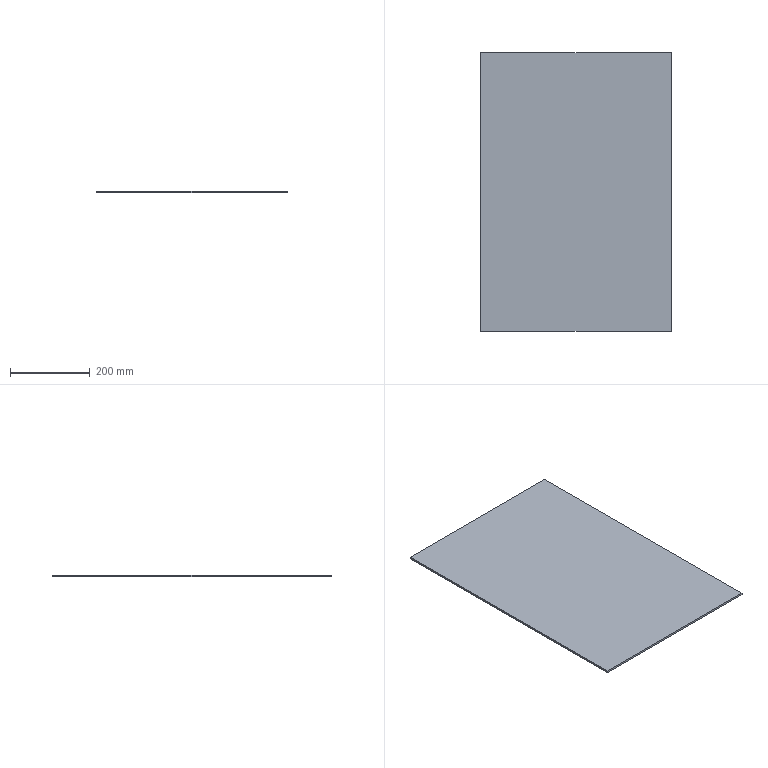Part | STEP file | 001-002-Face Plate-2 | 1 solid | 6 faces | box 478 x 698 x 5 mm | volume 1668220 mm3 | plane 6
STEP:
#1=CARTESIAN_POINT('',(0.,0.,0.));
#2=DIRECTION('',(0.,0.,1.));
#3=DIRECTION('',(1.,0.,0.));
#4=AXIS2_PLACEMENT_3D('',#1,#2,#3);
#5=CARTESIAN_POINT('',(239.,-349.,0.));
#6=VERTEX_POINT('',#5);
#7=CARTESIAN_POINT('',(239.,349.,0.));
#8=VERTEX_POINT('',#7);
#9=CARTESIAN_POINT('',(239.,-349.,0.));
#10=DIRECTION('',(0.,1.,0.));
#11=VECTOR('',#10,1.);
#12=LINE('',#9,#11);
#13=CARTESIAN_POINT('',(239.,-349.,5.));
#14=DIRECTION('',(-1.,0.,0.));
#15=DIRECTION('',(0.,0.,1.));
#16=AXIS2_PLACEMENT_3D('',#13,#14,#15);
#17=PLANE('',#16);
#18=CARTESIAN_POINT('',(-5.,0.));
#19=DIRECTION('',(0.,1.));
#20=VECTOR('',#19,1.);
#21=LINE('',#18,#20);
#22=(GEOMETRIC_REPRESENTATION_CONTEXT(2)PARAMETRIC_REPRESENTATION_CONTEXT()REPRESENTATION_CONTEXT('',''));
#23=DEFINITIONAL_REPRESENTATION('',(#21),#22);
#24=PCURVE('',#17,#23);
#25=CARTESIAN_POINT('',(0.,0.,0.));
#26=DIRECTION('',(0.,0.,-1.));
#27=DIRECTION('',(-1.,0.,0.));
#28=AXIS2_PLACEMENT_3D('',#25,#26,#27);
#29=PLANE('',#28);
#30=CARTESIAN_POINT('',(-239.,-349.));
#31=DIRECTION('',(0.,1.));
#32=VECTOR('',#31,1.);
#33=LINE('',#30,#32);
#34=(GEOMETRIC_REPRESENTATION_CONTEXT(2)PARAMETRIC_REPRESENTATION_CONTEXT()REPRESENTATION_CONTEXT('',''));
#35=DEFINITIONAL_REPRESENTATION('',(#33),#34);
#36=PCURVE('',#29,#35);
#37=SURFACE_CURVE('',#12,(#24,#36),.PCURVE_S1.);
#38=EDGE_CURVE('',#6,#8,#37,.T.);
#39=ORIENTED_EDGE('',*,*,#38,.T.);
#40=CARTESIAN_POINT('',(239.,349.,5.));
#41=VERTEX_POINT('',#40);
#42=CARTESIAN_POINT('',(239.,349.,5.));
#43=DIRECTION('',(0.,0.,-1.));
#44=VECTOR('',#43,1.);
#45=LINE('',#42,#44);
#46=CARTESIAN_POINT('',(0.,698.));
#47=DIRECTION('',(-1.,0.));
#48=VECTOR('',#47,1.);
#49=LINE('',#46,#48);
#50=(GEOMETRIC_REPRESENTATION_CONTEXT(2)PARAMETRIC_REPRESENTATION_CONTEXT()REPRESENTATION_CONTEXT('',''));
#51=DEFINITIONAL_REPRESENTATION('',(#49),#50);
#52=PCURVE('',#17,#51);
#53=CARTESIAN_POINT('',(-239.,349.,5.));
#54=DIRECTION('',(0.,-1.,0.));
#55=DIRECTION('',(0.,0.,-1.));
#56=AXIS2_PLACEMENT_3D('',#53,#54,#55);
#57=PLANE('',#56);
#58=CARTESIAN_POINT('',(0.,478.));
#59=DIRECTION('',(1.,0.));
#60=VECTOR('',#59,1.);
#61=LINE('',#58,#60);
#62=(GEOMETRIC_REPRESENTATION_CONTEXT(2)PARAMETRIC_REPRESENTATION_CONTEXT()REPRESENTATION_CONTEXT('',''));
#63=DEFINITIONAL_REPRESENTATION('',(#61),#62);
#64=PCURVE('',#57,#63);
#65=SURFACE_CURVE('',#45,(#52,#64),.PCURVE_S1.);
#66=EDGE_CURVE('',#41,#8,#65,.T.);
#67=ORIENTED_EDGE('',*,*,#66,.F.);
#68=CARTESIAN_POINT('',(239.,-349.,5.));
#69=VERTEX_POINT('',#68);
#70=CARTESIAN_POINT('',(239.,-349.,5.));
#71=DIRECTION('',(0.,1.,0.));
#72=VECTOR('',#71,1.);
#73=LINE('',#70,#72);
#74=CARTESIAN_POINT('',(0.,0.));
#75=DIRECTION('',(0.,1.));
#76=VECTOR('',#75,1.);
#77=LINE('',#74,#76);
#78=(GEOMETRIC_REPRESENTATION_CONTEXT(2)PARAMETRIC_REPRESENTATION_CONTEXT()REPRESENTATION_CONTEXT('',''));
#79=DEFINITIONAL_REPRESENTATION('',(#77),#78);
#80=PCURVE('',#17,#79);
#81=CARTESIAN_POINT('',(0.,0.,5.));
#82=DIRECTION('',(0.,0.,-1.));
#83=DIRECTION('',(-1.,0.,0.));
#84=AXIS2_PLACEMENT_3D('',#81,#82,#83);
#85=PLANE('',#84);
#86=CARTESIAN_POINT('',(-239.,-349.));
#87=DIRECTION('',(0.,1.));
#88=VECTOR('',#87,1.);
#89=LINE('',#86,#88);
#90=(GEOMETRIC_REPRESENTATION_CONTEXT(2)PARAMETRIC_REPRESENTATION_CONTEXT()REPRESENTATION_CONTEXT('',''));
#91=DEFINITIONAL_REPRESENTATION('',(#89),#90);
#92=PCURVE('',#85,#91);
#93=SURFACE_CURVE('',#73,(#80,#92),.PCURVE_S1.);
#94=EDGE_CURVE('',#69,#41,#93,.T.);
#95=ORIENTED_EDGE('',*,*,#94,.F.);
#96=CARTESIAN_POINT('',(239.,-349.,5.));
#97=DIRECTION('',(0.,0.,-1.));
#98=VECTOR('',#97,1.);
#99=LINE('',#96,#98);
#100=CARTESIAN_POINT('',(0.,0.));
#101=DIRECTION('',(-1.,0.));
#102=VECTOR('',#101,1.);
#103=LINE('',#100,#102);
#104=(GEOMETRIC_REPRESENTATION_CONTEXT(2)PARAMETRIC_REPRESENTATION_CONTEXT()REPRESENTATION_CONTEXT('',''));
#105=DEFINITIONAL_REPRESENTATION('',(#103),#104);
#106=PCURVE('',#17,#105);
#107=CARTESIAN_POINT('',(-239.,-349.,5.));
#108=DIRECTION('',(0.,1.,0.));
#109=DIRECTION('',(0.,0.,1.));
#110=AXIS2_PLACEMENT_3D('',#107,#108,#109);
#111=PLANE('',#110);
#112=CARTESIAN_POINT('',(0.,478.));
#113=DIRECTION('',(-1.,0.));
#114=VECTOR('',#113,1.);
#115=LINE('',#112,#114);
#116=(GEOMETRIC_REPRESENTATION_CONTEXT(2)PARAMETRIC_REPRESENTATION_CONTEXT()REPRESENTATION_CONTEXT('',''));
#117=DEFINITIONAL_REPRESENTATION('',(#115),#116);
#118=PCURVE('',#111,#117);
#119=SURFACE_CURVE('',#99,(#106,#118),.PCURVE_S1.);
#120=EDGE_CURVE('',#69,#6,#119,.T.);
#121=ORIENTED_EDGE('',*,*,#120,.T.);
#122=EDGE_LOOP('',(#39,#67,#95,#121));
#123=FACE_BOUND('',#122,.T.);
#124=ADVANCED_FACE('',(#123),#17,.F.);
#125=CARTESIAN_POINT('',(-239.,349.,0.));
#126=VERTEX_POINT('',#125);
#127=CARTESIAN_POINT('',(-239.,349.,0.));
#128=DIRECTION('',(-1.,0.,0.));
#129=VECTOR('',#128,1.);
#130=LINE('',#127,#129);
#131=CARTESIAN_POINT('',(5.,0.));
#132=DIRECTION('',(0.,-1.));
#133=VECTOR('',#132,1.);
#134=LINE('',#131,#133);
#135=(GEOMETRIC_REPRESENTATION_CONTEXT(2)PARAMETRIC_REPRESENTATION_CONTEXT()REPRESENTATION_CONTEXT('',''));
#136=DEFINITIONAL_REPRESENTATION('',(#134),#135);
#137=PCURVE('',#57,#136);
#138=CARTESIAN_POINT('',(239.,349.));
#139=DIRECTION('',(1.,0.));
#140=VECTOR('',#139,1.);
#141=LINE('',#138,#140);
#142=(GEOMETRIC_REPRESENTATION_CONTEXT(2)PARAMETRIC_REPRESENTATION_CONTEXT()REPRESENTATION_CONTEXT('',''));
#143=DEFINITIONAL_REPRESENTATION('',(#141),#142);
#144=PCURVE('',#29,#143);
#145=SURFACE_CURVE('',#130,(#137,#144),.PCURVE_S1.);
#146=EDGE_CURVE('',#8,#126,#145,.T.);
#147=ORIENTED_EDGE('',*,*,#146,.T.);
#148=CARTESIAN_POINT('',(-239.,349.,5.));
#149=VERTEX_POINT('',#148);
#150=CARTESIAN_POINT('',(-239.,349.,5.));
#151=DIRECTION('',(0.,0.,-1.));
#152=VECTOR('',#151,1.);
#153=LINE('',#150,#152);
#154=CARTESIAN_POINT('',(0.,0.));
#155=DIRECTION('',(1.,0.));
#156=VECTOR('',#155,1.);
#157=LINE('',#154,#156);
#158=(GEOMETRIC_REPRESENTATION_CONTEXT(2)PARAMETRIC_REPRESENTATION_CONTEXT()REPRESENTATION_CONTEXT('',''));
#159=DEFINITIONAL_REPRESENTATION('',(#157),#158);
#160=PCURVE('',#57,#159);
#161=CARTESIAN_POINT('',(-239.,-349.,5.));
#162=DIRECTION('',(1.,0.,0.));
#163=DIRECTION('',(0.,0.,-1.));
#164=AXIS2_PLACEMENT_3D('',#161,#162,#163);
#165=PLANE('',#164);
#166=CARTESIAN_POINT('',(0.,698.));
#167=DIRECTION('',(1.,0.));
#168=VECTOR('',#167,1.);
#169=LINE('',#166,#168);
#170=(GEOMETRIC_REPRESENTATION_CONTEXT(2)PARAMETRIC_REPRESENTATION_CONTEXT()REPRESENTATION_CONTEXT('',''));
#171=DEFINITIONAL_REPRESENTATION('',(#169),#170);
#172=PCURVE('',#165,#171);
#173=SURFACE_CURVE('',#153,(#160,#172),.PCURVE_S1.);
#174=EDGE_CURVE('',#149,#126,#173,.T.);
#175=ORIENTED_EDGE('',*,*,#174,.F.);
#176=CARTESIAN_POINT('',(-239.,349.,5.));
#177=DIRECTION('',(-1.,0.,0.));
#178=VECTOR('',#177,1.);
#179=LINE('',#176,#178);
#180=CARTESIAN_POINT('',(0.,0.));
#181=DIRECTION('',(0.,-1.));
#182=VECTOR('',#181,1.);
#183=LINE('',#180,#182);
#184=(GEOMETRIC_REPRESENTATION_CONTEXT(2)PARAMETRIC_REPRESENTATION_CONTEXT()REPRESENTATION_CONTEXT('',''));
#185=DEFINITIONAL_REPRESENTATION('',(#183),#184);
#186=PCURVE('',#57,#185);
#187=CARTESIAN_POINT('',(239.,349.));
#188=DIRECTION('',(1.,0.));
#189=VECTOR('',#188,1.);
#190=LINE('',#187,#189);
#191=(GEOMETRIC_REPRESENTATION_CONTEXT(2)PARAMETRIC_REPRESENTATION_CONTEXT()REPRESENTATION_CONTEXT('',''));
#192=DEFINITIONAL_REPRESENTATION('',(#190),#191);
#193=PCURVE('',#85,#192);
#194=SURFACE_CURVE('',#179,(#186,#193),.PCURVE_S1.);
#195=EDGE_CURVE('',#41,#149,#194,.T.);
#196=ORIENTED_EDGE('',*,*,#195,.F.);
#197=ORIENTED_EDGE('',*,*,#66,.T.);
#198=EDGE_LOOP('',(#147,#175,#196,#197));
#199=FACE_BOUND('',#198,.T.);
#200=ADVANCED_FACE('',(#199),#57,.F.);
#201=CARTESIAN_POINT('',(-239.,-349.,0.));
#202=VERTEX_POINT('',#201);
#203=CARTESIAN_POINT('',(-239.,-349.,0.));
#204=DIRECTION('',(0.,-1.,0.));
#205=VECTOR('',#204,1.);
#206=LINE('',#203,#205);
#207=CARTESIAN_POINT('',(5.,0.));
#208=DIRECTION('',(0.,-1.));
#209=VECTOR('',#208,1.);
#210=LINE('',#207,#209);
#211=(GEOMETRIC_REPRESENTATION_CONTEXT(2)PARAMETRIC_REPRESENTATION_CONTEXT()REPRESENTATION_CONTEXT('',''));
#212=DEFINITIONAL_REPRESENTATION('',(#210),#211);
#213=PCURVE('',#165,#212);
#214=CARTESIAN_POINT('',(239.,-349.));
#215=DIRECTION('',(0.,-1.));
#216=VECTOR('',#215,1.);
#217=LINE('',#214,#216);
#218=(GEOMETRIC_REPRESENTATION_CONTEXT(2)PARAMETRIC_REPRESENTATION_CONTEXT()REPRESENTATION_CONTEXT('',''));
#219=DEFINITIONAL_REPRESENTATION('',(#217),#218);
#220=PCURVE('',#29,#219);
#221=SURFACE_CURVE('',#206,(#213,#220),.PCURVE_S1.);
#222=EDGE_CURVE('',#126,#202,#221,.T.);
#223=ORIENTED_EDGE('',*,*,#222,.T.);
#224=CARTESIAN_POINT('',(-239.,-349.,5.));
#225=VERTEX_POINT('',#224);
#226=CARTESIAN_POINT('',(-239.,-349.,5.));
#227=DIRECTION('',(0.,0.,-1.));
#228=VECTOR('',#227,1.);
#229=LINE('',#226,#228);
#230=CARTESIAN_POINT('',(0.,0.));
#231=DIRECTION('',(1.,0.));
#232=VECTOR('',#231,1.);
#233=LINE('',#230,#232);
#234=(GEOMETRIC_REPRESENTATION_CONTEXT(2)PARAMETRIC_REPRESENTATION_CONTEXT()REPRESENTATION_CONTEXT('',''));
#235=DEFINITIONAL_REPRESENTATION('',(#233),#234);
#236=PCURVE('',#165,#235);
#237=CARTESIAN_POINT('',(0.,0.));
#238=DIRECTION('',(-1.,0.));
#239=VECTOR('',#238,1.);
#240=LINE('',#237,#239);
#241=(GEOMETRIC_REPRESENTATION_CONTEXT(2)PARAMETRIC_REPRESENTATION_CONTEXT()REPRESENTATION_CONTEXT('',''));
#242=DEFINITIONAL_REPRESENTATION('',(#240),#241);
#243=PCURVE('',#111,#242);
#244=SURFACE_CURVE('',#229,(#236,#243),.PCURVE_S1.);
#245=EDGE_CURVE('',#225,#202,#244,.T.);
#246=ORIENTED_EDGE('',*,*,#245,.F.);
#247=CARTESIAN_POINT('',(-239.,-349.,5.));
#248=DIRECTION('',(0.,-1.,0.));
#249=VECTOR('',#248,1.);
#250=LINE('',#247,#249);
#251=CARTESIAN_POINT('',(0.,0.));
#252=DIRECTION('',(0.,-1.));
#253=VECTOR('',#252,1.);
#254=LINE('',#251,#253);
#255=(GEOMETRIC_REPRESENTATION_CONTEXT(2)PARAMETRIC_REPRESENTATION_CONTEXT()REPRESENTATION_CONTEXT('',''));
#256=DEFINITIONAL_REPRESENTATION('',(#254),#255);
#257=PCURVE('',#165,#256);
#258=CARTESIAN_POINT('',(239.,-349.));
#259=DIRECTION('',(0.,-1.));
#260=VECTOR('',#259,1.);
#261=LINE('',#258,#260);
#262=(GEOMETRIC_REPRESENTATION_CONTEXT(2)PARAMETRIC_REPRESENTATION_CONTEXT()REPRESENTATION_CONTEXT('',''));
#263=DEFINITIONAL_REPRESENTATION('',(#261),#262);
#264=PCURVE('',#85,#263);
#265=SURFACE_CURVE('',#250,(#257,#264),.PCURVE_S1.);
#266=EDGE_CURVE('',#149,#225,#265,.T.);
#267=ORIENTED_EDGE('',*,*,#266,.F.);
#268=ORIENTED_EDGE('',*,*,#174,.T.);
#269=EDGE_LOOP('',(#223,#246,#267,#268));
#270=FACE_BOUND('',#269,.T.);
#271=ADVANCED_FACE('',(#270),#165,.F.);
#272=CARTESIAN_POINT('',(-239.,-349.,0.));
#273=DIRECTION('',(1.,0.,0.));
#274=VECTOR('',#273,1.);
#275=LINE('',#272,#274);
#276=CARTESIAN_POINT('',(-5.,0.));
#277=DIRECTION('',(0.,1.));
#278=VECTOR('',#277,1.);
#279=LINE('',#276,#278);
#280=(GEOMETRIC_REPRESENTATION_CONTEXT(2)PARAMETRIC_REPRESENTATION_CONTEXT()REPRESENTATION_CONTEXT('',''));
#281=DEFINITIONAL_REPRESENTATION('',(#279),#280);
#282=PCURVE('',#111,#281);
#283=CARTESIAN_POINT('',(239.,-349.));
#284=DIRECTION('',(-1.,0.));
#285=VECTOR('',#284,1.);
#286=LINE('',#283,#285);
#287=(GEOMETRIC_REPRESENTATION_CONTEXT(2)PARAMETRIC_REPRESENTATION_CONTEXT()REPRESENTATION_CONTEXT('',''));
#288=DEFINITIONAL_REPRESENTATION('',(#286),#287);
#289=PCURVE('',#29,#288);
#290=SURFACE_CURVE('',#275,(#282,#289),.PCURVE_S1.);
#291=EDGE_CURVE('',#202,#6,#290,.T.);
#292=ORIENTED_EDGE('',*,*,#291,.T.);
#293=ORIENTED_EDGE('',*,*,#120,.F.);
#294=CARTESIAN_POINT('',(-239.,-349.,5.));
#295=DIRECTION('',(1.,0.,0.));
#296=VECTOR('',#295,1.);
#297=LINE('',#294,#296);
#298=CARTESIAN_POINT('',(0.,0.));
#299=DIRECTION('',(0.,1.));
#300=VECTOR('',#299,1.);
#301=LINE('',#298,#300);
#302=(GEOMETRIC_REPRESENTATION_CONTEXT(2)PARAMETRIC_REPRESENTATION_CONTEXT()REPRESENTATION_CONTEXT('',''));
#303=DEFINITIONAL_REPRESENTATION('',(#301),#302);
#304=PCURVE('',#111,#303);
#305=CARTESIAN_POINT('',(239.,-349.));
#306=DIRECTION('',(-1.,0.));
#307=VECTOR('',#306,1.);
#308=LINE('',#305,#307);
#309=(GEOMETRIC_REPRESENTATION_CONTEXT(2)PARAMETRIC_REPRESENTATION_CONTEXT()REPRESENTATION_CONTEXT('',''));
#310=DEFINITIONAL_REPRESENTATION('',(#308),#309);
#311=PCURVE('',#85,#310);
#312=SURFACE_CURVE('',#297,(#304,#311),.PCURVE_S1.);
#313=EDGE_CURVE('',#225,#69,#312,.T.);
#314=ORIENTED_EDGE('',*,*,#313,.F.);
#315=ORIENTED_EDGE('',*,*,#245,.T.);
#316=EDGE_LOOP('',(#292,#293,#314,#315));
#317=FACE_BOUND('',#316,.T.);
#318=ADVANCED_FACE('',(#317),#111,.F.);
#319=ORIENTED_EDGE('',*,*,#94,.T.);
#320=ORIENTED_EDGE('',*,*,#195,.T.);
#321=ORIENTED_EDGE('',*,*,#266,.T.);
#322=ORIENTED_EDGE('',*,*,#313,.T.);
#323=EDGE_LOOP('',(#319,#320,#321,#322));
#324=FACE_BOUND('',#323,.T.);
#325=ADVANCED_FACE('',(#324),#85,.F.);
#326=ORIENTED_EDGE('',*,*,#38,.F.);
#327=ORIENTED_EDGE('',*,*,#291,.F.);
#328=ORIENTED_EDGE('',*,*,#222,.F.);
#329=ORIENTED_EDGE('',*,*,#146,.F.);
#330=EDGE_LOOP('',(#326,#327,#328,#329));
#331=FACE_BOUND('',#330,.T.);
#332=ADVANCED_FACE('',(#331),#29,.T.);
#333=CLOSED_SHELL('',(#124,#200,#271,#318,#325,#332));
#334=MANIFOLD_SOLID_BREP('',#333);
#335=(LENGTH_UNIT()NAMED_UNIT(*)SI_UNIT(.MILLI.,.METRE.));
#336=UNCERTAINTY_MEASURE_WITH_UNIT(LENGTH_MEASURE(0.0000001),#335,'','');
#337=(NAMED_UNIT(*)PLANE_ANGLE_UNIT()SI_UNIT($,.RADIAN.));
#338=(NAMED_UNIT(*)SI_UNIT($,.STERADIAN.)SOLID_ANGLE_UNIT());
#339=(GEOMETRIC_REPRESENTATION_CONTEXT(3)GLOBAL_UNCERTAINTY_ASSIGNED_CONTEXT((#336))GLOBAL_UNIT_ASSIGNED_CONTEXT((#335,#337,#338))REPRESENTATION_CONTEXT('',''));
#340=ADVANCED_BREP_SHAPE_REPRESENTATION('',(#4,#334),#339);